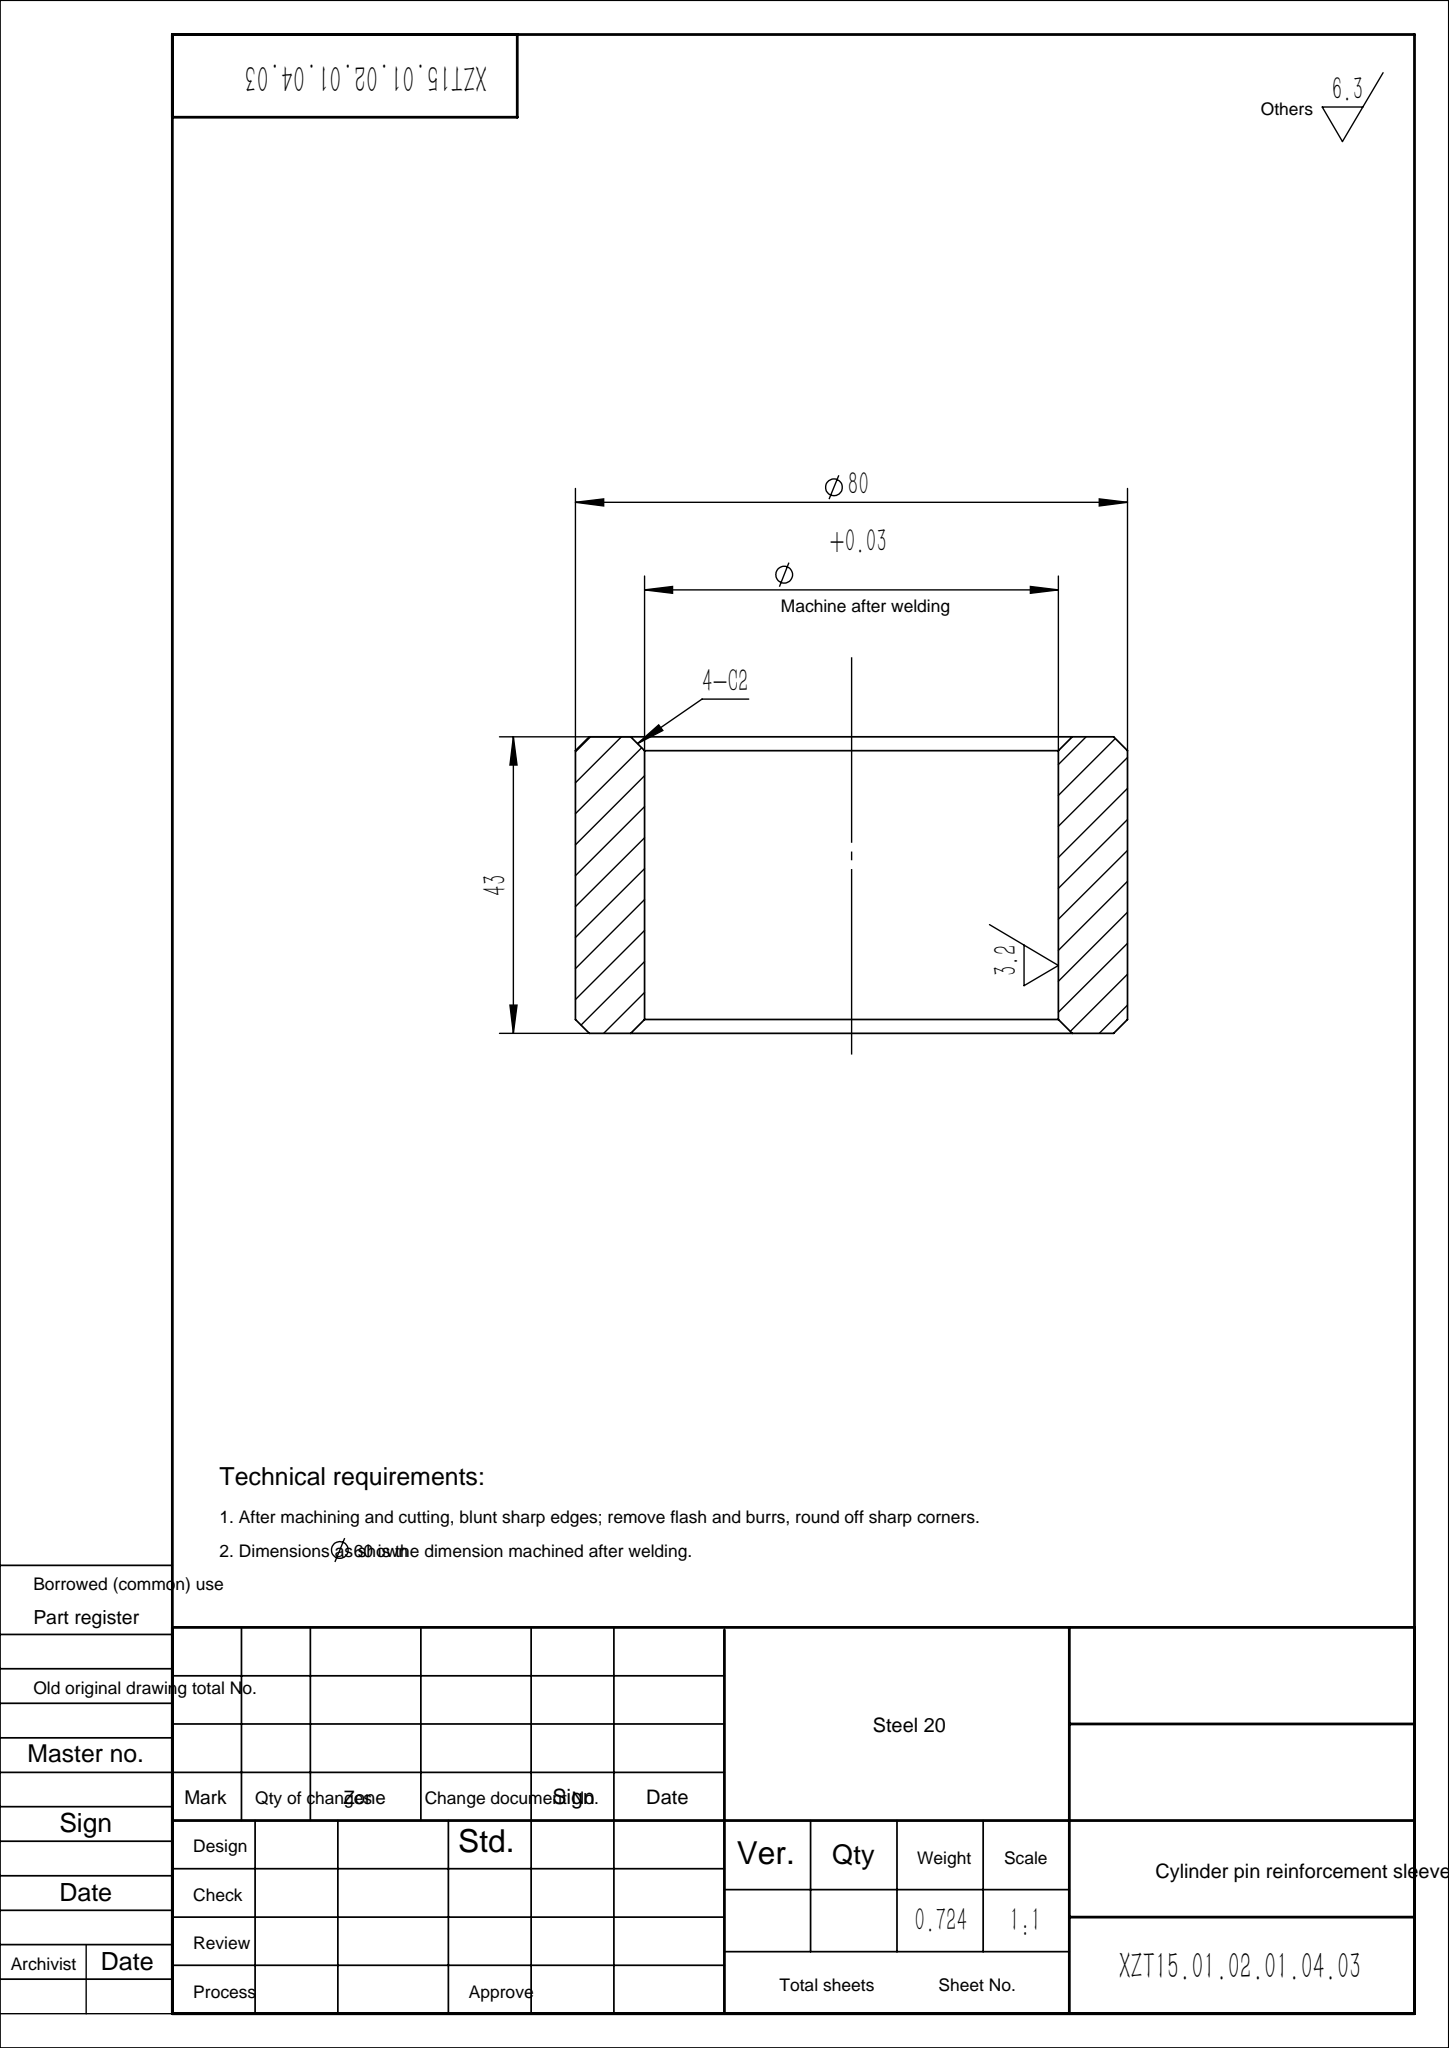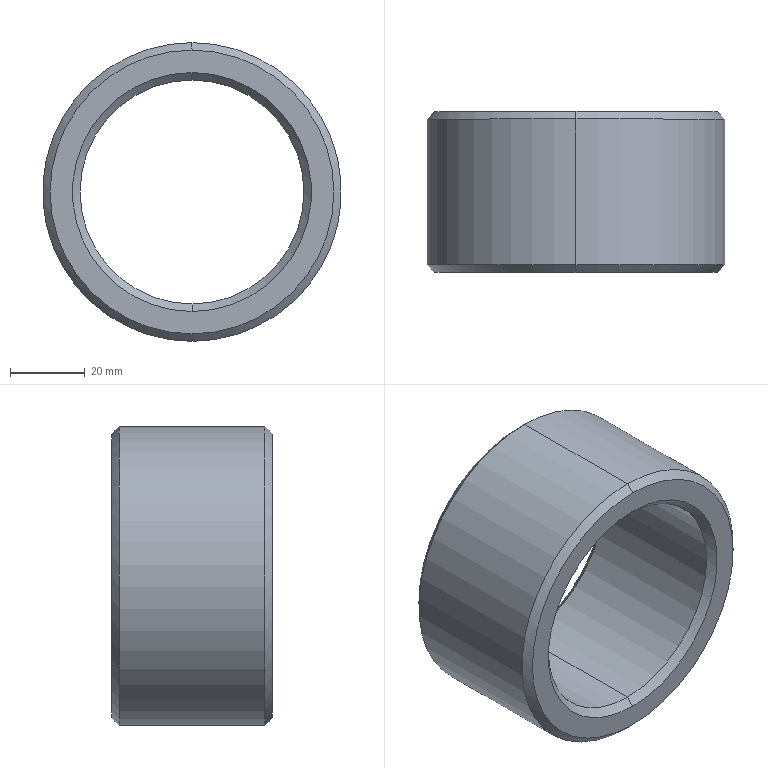Part | SolidWorks | features Chamfer 1, Extrusion 1 | 1 solid | 14 faces | box 80 x 43 x 80 mm | volume 92803 mm3 | cone 8 | cylinder 4 | plane 2 | commonest cylinder face diameters 60 x2 80 x2
STEP:
#1=CARTESIAN_POINT('',(0.,43.,38.));
#2=VERTEX_POINT('',#1);
#3=CARTESIAN_POINT('',(0.,43.,-38.));
#4=VERTEX_POINT('',#3);
#5=CARTESIAN_POINT('',(0.,43.,0.));
#6=DIRECTION('',(0.,1.,0.));
#7=DIRECTION('',(0.,0.,1.));
#8=AXIS2_PLACEMENT_3D('',#5,#6,#7);
#9=CIRCLE('',#8,38.);
#10=EDGE_CURVE('',#2,#4,#9,.T.);
#11=ORIENTED_EDGE('',*,*,#10,.F.);
#12=CARTESIAN_POINT('',(0.,41.,40.));
#13=VERTEX_POINT('',#12);
#14=CARTESIAN_POINT('',(0.,43.,38.));
#15=DIRECTION('',(0.,-0.7071,0.7071));
#16=VECTOR('',#15,1000.);
#17=LINE('',#14,#16);
#18=EDGE_CURVE('',#2,#13,#17,.T.);
#19=ORIENTED_EDGE('',*,*,#18,.T.);
#20=CARTESIAN_POINT('',(0.,41.,-40.));
#21=VERTEX_POINT('',#20);
#22=CARTESIAN_POINT('',(0.,41.,0.));
#23=DIRECTION('',(0.,-1.,0.));
#24=DIRECTION('',(0.,0.,1.));
#25=AXIS2_PLACEMENT_3D('',#22,#23,#24);
#26=CIRCLE('',#25,40.);
#27=EDGE_CURVE('',#21,#13,#26,.T.);
#28=ORIENTED_EDGE('',*,*,#27,.F.);
#29=CARTESIAN_POINT('',(0.,43.,-38.));
#30=DIRECTION('',(0.,-0.7071,-0.7071));
#31=VECTOR('',#30,1000.);
#32=LINE('',#29,#31);
#33=EDGE_CURVE('',#4,#21,#32,.T.);
#34=ORIENTED_EDGE('',*,*,#33,.F.);
#35=EDGE_LOOP('',(#11,#19,#28,#34));
#36=FACE_OUTER_BOUND('',#35,.T.);
#37=CARTESIAN_POINT('',(0.,43.,0.));
#38=DIRECTION('',(0.,-1.,0.));
#39=DIRECTION('',(0.,0.,-1.));
#40=AXIS2_PLACEMENT_3D('',#37,#38,#39);
#41=CONICAL_SURFACE('',#40,38.,0.7854);
#42=ADVANCED_FACE('',(#36),#41,.T.);
#43=CARTESIAN_POINT('',(0.,0.,-38.));
#44=VERTEX_POINT('',#43);
#45=CARTESIAN_POINT('',(0.,0.,38.));
#46=VERTEX_POINT('',#45);
#47=CARTESIAN_POINT('',(0.,0.,0.));
#48=DIRECTION('',(0.,-1.,0.));
#49=DIRECTION('',(0.,0.,1.));
#50=AXIS2_PLACEMENT_3D('',#47,#48,#49);
#51=CIRCLE('',#50,38.);
#52=EDGE_CURVE('',#44,#46,#51,.T.);
#53=ORIENTED_EDGE('',*,*,#52,.F.);
#54=CARTESIAN_POINT('',(0.,2.,-40.));
#55=VERTEX_POINT('',#54);
#56=CARTESIAN_POINT('',(0.,2.,-40.));
#57=DIRECTION('',(0.,0.7071,-0.7071));
#58=VECTOR('',#57,1000.);
#59=LINE('',#56,#58);
#60=EDGE_CURVE('',#44,#55,#59,.T.);
#61=ORIENTED_EDGE('',*,*,#60,.T.);
#62=CARTESIAN_POINT('',(0.,2.,40.));
#63=VERTEX_POINT('',#62);
#64=CARTESIAN_POINT('',(0.,2.,0.));
#65=DIRECTION('',(0.,1.,0.));
#66=DIRECTION('',(0.,0.,1.));
#67=AXIS2_PLACEMENT_3D('',#64,#65,#66);
#68=CIRCLE('',#67,40.);
#69=EDGE_CURVE('',#63,#55,#68,.T.);
#70=ORIENTED_EDGE('',*,*,#69,.F.);
#71=CARTESIAN_POINT('',(0.,2.,40.));
#72=DIRECTION('',(0.,0.7071,0.7071));
#73=VECTOR('',#72,1000.);
#74=LINE('',#71,#73);
#75=EDGE_CURVE('',#46,#63,#74,.T.);
#76=ORIENTED_EDGE('',*,*,#75,.F.);
#77=EDGE_LOOP('',(#53,#61,#70,#76));
#78=FACE_OUTER_BOUND('',#77,.T.);
#79=CARTESIAN_POINT('',(0.,2.,0.));
#80=DIRECTION('',(0.,1.,0.));
#81=DIRECTION('',(0.,0.,1.));
#82=AXIS2_PLACEMENT_3D('',#79,#80,#81);
#83=CONICAL_SURFACE('',#82,40.,0.7854);
#84=ADVANCED_FACE('',(#78),#83,.T.);
#85=CARTESIAN_POINT('',(0.,41.,-30.));
#86=VERTEX_POINT('',#85);
#87=CARTESIAN_POINT('',(0.,41.,30.));
#88=VERTEX_POINT('',#87);
#89=CARTESIAN_POINT('',(0.,41.,0.));
#90=DIRECTION('',(0.,1.,0.));
#91=DIRECTION('',(0.,0.,1.));
#92=AXIS2_PLACEMENT_3D('',#89,#90,#91);
#93=CIRCLE('',#92,30.);
#94=EDGE_CURVE('',#86,#88,#93,.T.);
#95=ORIENTED_EDGE('',*,*,#94,.F.);
#96=CARTESIAN_POINT('',(0.,43.,-32.));
#97=VERTEX_POINT('',#96);
#98=CARTESIAN_POINT('',(0.,41.,-30.));
#99=DIRECTION('',(0.,0.7071,-0.7071));
#100=VECTOR('',#99,1000.);
#101=LINE('',#98,#100);
#102=EDGE_CURVE('',#86,#97,#101,.T.);
#103=ORIENTED_EDGE('',*,*,#102,.T.);
#104=CARTESIAN_POINT('',(0.,43.,32.));
#105=VERTEX_POINT('',#104);
#106=CARTESIAN_POINT('',(0.,43.,0.));
#107=DIRECTION('',(0.,-1.,0.));
#108=DIRECTION('',(0.,0.,1.));
#109=AXIS2_PLACEMENT_3D('',#106,#107,#108);
#110=CIRCLE('',#109,32.);
#111=EDGE_CURVE('',#105,#97,#110,.T.);
#112=ORIENTED_EDGE('',*,*,#111,.F.);
#113=CARTESIAN_POINT('',(0.,41.,30.));
#114=DIRECTION('',(0.,0.7071,0.7071));
#115=VECTOR('',#114,1000.);
#116=LINE('',#113,#115);
#117=EDGE_CURVE('',#88,#105,#116,.T.);
#118=ORIENTED_EDGE('',*,*,#117,.F.);
#119=EDGE_LOOP('',(#95,#103,#112,#118));
#120=FACE_OUTER_BOUND('',#119,.T.);
#121=CARTESIAN_POINT('',(0.,41.,0.));
#122=DIRECTION('',(0.,1.,0.));
#123=DIRECTION('',(0.,0.,1.));
#124=AXIS2_PLACEMENT_3D('',#121,#122,#123);
#125=CONICAL_SURFACE('',#124,30.,0.7854);
#126=ADVANCED_FACE('',(#120),#125,.F.);
#127=CARTESIAN_POINT('',(0.,2.,30.));
#128=VERTEX_POINT('',#127);
#129=CARTESIAN_POINT('',(0.,2.,-30.));
#130=VERTEX_POINT('',#129);
#131=CARTESIAN_POINT('',(0.,2.,0.));
#132=DIRECTION('',(0.,-1.,0.));
#133=DIRECTION('',(0.,0.,1.));
#134=AXIS2_PLACEMENT_3D('',#131,#132,#133);
#135=CIRCLE('',#134,30.);
#136=EDGE_CURVE('',#128,#130,#135,.T.);
#137=ORIENTED_EDGE('',*,*,#136,.F.);
#138=CARTESIAN_POINT('',(0.,0.,32.));
#139=VERTEX_POINT('',#138);
#140=CARTESIAN_POINT('',(0.,0.,32.));
#141=DIRECTION('',(0.,-0.7071,0.7071));
#142=VECTOR('',#141,1000.);
#143=LINE('',#140,#142);
#144=EDGE_CURVE('',#128,#139,#143,.T.);
#145=ORIENTED_EDGE('',*,*,#144,.T.);
#146=CARTESIAN_POINT('',(0.,0.,-32.));
#147=VERTEX_POINT('',#146);
#148=CARTESIAN_POINT('',(0.,0.,0.));
#149=DIRECTION('',(0.,1.,0.));
#150=DIRECTION('',(0.,0.,1.));
#151=AXIS2_PLACEMENT_3D('',#148,#149,#150);
#152=CIRCLE('',#151,32.);
#153=EDGE_CURVE('',#147,#139,#152,.T.);
#154=ORIENTED_EDGE('',*,*,#153,.F.);
#155=CARTESIAN_POINT('',(0.,0.,-32.));
#156=DIRECTION('',(0.,-0.7071,-0.7071));
#157=VECTOR('',#156,1000.);
#158=LINE('',#155,#157);
#159=EDGE_CURVE('',#130,#147,#158,.T.);
#160=ORIENTED_EDGE('',*,*,#159,.F.);
#161=EDGE_LOOP('',(#137,#145,#154,#160));
#162=FACE_OUTER_BOUND('',#161,.T.);
#163=CARTESIAN_POINT('',(0.,0.,0.));
#164=DIRECTION('',(0.,-1.,0.));
#165=DIRECTION('',(0.,0.,-1.));
#166=AXIS2_PLACEMENT_3D('',#163,#164,#165);
#167=CONICAL_SURFACE('',#166,32.,0.7854);
#168=ADVANCED_FACE('',(#162),#167,.F.);
#169=ORIENTED_EDGE('',*,*,#94,.T.);
#170=CARTESIAN_POINT('',(0.,43.,30.));
#171=DIRECTION('',(0.,-1.,0.));
#172=VECTOR('',#171,1000.);
#173=LINE('',#170,#172);
#174=EDGE_CURVE('',#88,#128,#173,.T.);
#175=ORIENTED_EDGE('',*,*,#174,.T.);
#176=ORIENTED_EDGE('',*,*,#136,.T.);
#177=CARTESIAN_POINT('',(0.,43.,-30.));
#178=DIRECTION('',(0.,-1.,0.));
#179=VECTOR('',#178,1000.);
#180=LINE('',#177,#179);
#181=EDGE_CURVE('',#86,#130,#180,.T.);
#182=ORIENTED_EDGE('',*,*,#181,.F.);
#183=EDGE_LOOP('',(#169,#175,#176,#182));
#184=FACE_OUTER_BOUND('',#183,.T.);
#185=CARTESIAN_POINT('',(0.,43.,0.));
#186=DIRECTION('',(0.,-1.,0.));
#187=DIRECTION('',(0.,0.,-1.));
#188=AXIS2_PLACEMENT_3D('',#185,#186,#187);
#189=CYLINDRICAL_SURFACE('',#188,30.);
#190=ADVANCED_FACE('',(#184),#189,.F.);
#191=ORIENTED_EDGE('',*,*,#27,.T.);
#192=CARTESIAN_POINT('',(0.,43.,40.));
#193=DIRECTION('',(0.,-1.,0.));
#194=VECTOR('',#193,1000.);
#195=LINE('',#192,#194);
#196=EDGE_CURVE('',#13,#63,#195,.T.);
#197=ORIENTED_EDGE('',*,*,#196,.T.);
#198=ORIENTED_EDGE('',*,*,#69,.T.);
#199=CARTESIAN_POINT('',(0.,43.,-40.));
#200=DIRECTION('',(0.,-1.,0.));
#201=VECTOR('',#200,1000.);
#202=LINE('',#199,#201);
#203=EDGE_CURVE('',#21,#55,#202,.T.);
#204=ORIENTED_EDGE('',*,*,#203,.F.);
#205=EDGE_LOOP('',(#191,#197,#198,#204));
#206=FACE_OUTER_BOUND('',#205,.T.);
#207=CARTESIAN_POINT('',(0.,43.,0.));
#208=DIRECTION('',(0.,-1.,0.));
#209=DIRECTION('',(0.,0.,-1.));
#210=AXIS2_PLACEMENT_3D('',#207,#208,#209);
#211=CYLINDRICAL_SURFACE('',#210,40.);
#212=ADVANCED_FACE('',(#206),#211,.T.);
#213=ORIENTED_EDGE('',*,*,#111,.T.);
#214=CARTESIAN_POINT('',(0.,43.,0.));
#215=DIRECTION('',(0.,-1.,0.));
#216=DIRECTION('',(0.,0.,1.));
#217=AXIS2_PLACEMENT_3D('',#214,#215,#216);
#218=CIRCLE('',#217,32.);
#219=EDGE_CURVE('',#97,#105,#218,.T.);
#220=ORIENTED_EDGE('',*,*,#219,.T.);
#221=EDGE_LOOP('',(#213,#220));
#222=FACE_BOUND('',#221,.T.);
#223=CARTESIAN_POINT('',(0.,43.,0.));
#224=DIRECTION('',(0.,1.,0.));
#225=DIRECTION('',(0.,0.,1.));
#226=AXIS2_PLACEMENT_3D('',#223,#224,#225);
#227=CIRCLE('',#226,38.);
#228=EDGE_CURVE('',#4,#2,#227,.T.);
#229=ORIENTED_EDGE('',*,*,#228,.T.);
#230=ORIENTED_EDGE('',*,*,#10,.T.);
#231=EDGE_LOOP('',(#229,#230));
#232=FACE_OUTER_BOUND('',#231,.T.);
#233=CARTESIAN_POINT('',(0.,43.,0.));
#234=DIRECTION('',(0.,1.,0.));
#235=DIRECTION('',(0.,0.,1.));
#236=AXIS2_PLACEMENT_3D('',#233,#234,#235);
#237=PLANE('',#236);
#238=ADVANCED_FACE('',(#222,#232),#237,.T.);
#239=ORIENTED_EDGE('',*,*,#153,.T.);
#240=CARTESIAN_POINT('',(0.,0.,0.));
#241=DIRECTION('',(0.,1.,0.));
#242=DIRECTION('',(0.,0.,1.));
#243=AXIS2_PLACEMENT_3D('',#240,#241,#242);
#244=CIRCLE('',#243,32.);
#245=EDGE_CURVE('',#139,#147,#244,.T.);
#246=ORIENTED_EDGE('',*,*,#245,.T.);
#247=EDGE_LOOP('',(#239,#246));
#248=FACE_BOUND('',#247,.T.);
#249=CARTESIAN_POINT('',(0.,0.,0.));
#250=DIRECTION('',(0.,-1.,0.));
#251=DIRECTION('',(0.,0.,1.));
#252=AXIS2_PLACEMENT_3D('',#249,#250,#251);
#253=CIRCLE('',#252,38.);
#254=EDGE_CURVE('',#46,#44,#253,.T.);
#255=ORIENTED_EDGE('',*,*,#254,.T.);
#256=ORIENTED_EDGE('',*,*,#52,.T.);
#257=EDGE_LOOP('',(#255,#256));
#258=FACE_OUTER_BOUND('',#257,.T.);
#259=CARTESIAN_POINT('',(0.,0.,0.));
#260=DIRECTION('',(0.,1.,0.));
#261=DIRECTION('',(0.,0.,1.));
#262=AXIS2_PLACEMENT_3D('',#259,#260,#261);
#263=PLANE('',#262);
#264=ADVANCED_FACE('',(#248,#258),#263,.F.);
#265=ORIENTED_EDGE('',*,*,#196,.F.);
#266=CARTESIAN_POINT('',(0.,41.,0.));
#267=DIRECTION('',(0.,-1.,0.));
#268=DIRECTION('',(0.,0.,1.));
#269=AXIS2_PLACEMENT_3D('',#266,#267,#268);
#270=CIRCLE('',#269,40.);
#271=EDGE_CURVE('',#13,#21,#270,.T.);
#272=ORIENTED_EDGE('',*,*,#271,.T.);
#273=ORIENTED_EDGE('',*,*,#203,.T.);
#274=CARTESIAN_POINT('',(0.,2.,0.));
#275=DIRECTION('',(0.,1.,0.));
#276=DIRECTION('',(0.,0.,1.));
#277=AXIS2_PLACEMENT_3D('',#274,#275,#276);
#278=CIRCLE('',#277,40.);
#279=EDGE_CURVE('',#55,#63,#278,.T.);
#280=ORIENTED_EDGE('',*,*,#279,.T.);
#281=EDGE_LOOP('',(#265,#272,#273,#280));
#282=FACE_OUTER_BOUND('',#281,.T.);
#283=CARTESIAN_POINT('',(0.,43.,0.));
#284=DIRECTION('',(0.,-1.,0.));
#285=DIRECTION('',(0.,0.,-1.));
#286=AXIS2_PLACEMENT_3D('',#283,#284,#285);
#287=CYLINDRICAL_SURFACE('',#286,40.);
#288=ADVANCED_FACE('',(#282),#287,.T.);
#289=ORIENTED_EDGE('',*,*,#174,.F.);
#290=CARTESIAN_POINT('',(0.,41.,0.));
#291=DIRECTION('',(0.,1.,0.));
#292=DIRECTION('',(0.,0.,1.));
#293=AXIS2_PLACEMENT_3D('',#290,#291,#292);
#294=CIRCLE('',#293,30.);
#295=EDGE_CURVE('',#88,#86,#294,.T.);
#296=ORIENTED_EDGE('',*,*,#295,.T.);
#297=ORIENTED_EDGE('',*,*,#181,.T.);
#298=CARTESIAN_POINT('',(0.,2.,0.));
#299=DIRECTION('',(0.,-1.,0.));
#300=DIRECTION('',(0.,0.,1.));
#301=AXIS2_PLACEMENT_3D('',#298,#299,#300);
#302=CIRCLE('',#301,30.);
#303=EDGE_CURVE('',#130,#128,#302,.T.);
#304=ORIENTED_EDGE('',*,*,#303,.T.);
#305=EDGE_LOOP('',(#289,#296,#297,#304));
#306=FACE_OUTER_BOUND('',#305,.T.);
#307=CARTESIAN_POINT('',(0.,43.,0.));
#308=DIRECTION('',(0.,-1.,0.));
#309=DIRECTION('',(0.,0.,-1.));
#310=AXIS2_PLACEMENT_3D('',#307,#308,#309);
#311=CYLINDRICAL_SURFACE('',#310,30.);
#312=ADVANCED_FACE('',(#306),#311,.F.);
#313=ORIENTED_EDGE('',*,*,#144,.F.);
#314=ORIENTED_EDGE('',*,*,#303,.F.);
#315=ORIENTED_EDGE('',*,*,#159,.T.);
#316=ORIENTED_EDGE('',*,*,#245,.F.);
#317=EDGE_LOOP('',(#313,#314,#315,#316));
#318=FACE_OUTER_BOUND('',#317,.T.);
#319=CARTESIAN_POINT('',(0.,0.,0.));
#320=DIRECTION('',(0.,-1.,0.));
#321=DIRECTION('',(0.,0.,-1.));
#322=AXIS2_PLACEMENT_3D('',#319,#320,#321);
#323=CONICAL_SURFACE('',#322,32.,0.7854);
#324=ADVANCED_FACE('',(#318),#323,.F.);
#325=ORIENTED_EDGE('',*,*,#102,.F.);
#326=ORIENTED_EDGE('',*,*,#295,.F.);
#327=ORIENTED_EDGE('',*,*,#117,.T.);
#328=ORIENTED_EDGE('',*,*,#219,.F.);
#329=EDGE_LOOP('',(#325,#326,#327,#328));
#330=FACE_OUTER_BOUND('',#329,.T.);
#331=CARTESIAN_POINT('',(0.,41.,0.));
#332=DIRECTION('',(0.,1.,0.));
#333=DIRECTION('',(0.,0.,1.));
#334=AXIS2_PLACEMENT_3D('',#331,#332,#333);
#335=CONICAL_SURFACE('',#334,30.,0.7854);
#336=ADVANCED_FACE('',(#330),#335,.F.);
#337=ORIENTED_EDGE('',*,*,#60,.F.);
#338=ORIENTED_EDGE('',*,*,#254,.F.);
#339=ORIENTED_EDGE('',*,*,#75,.T.);
#340=ORIENTED_EDGE('',*,*,#279,.F.);
#341=EDGE_LOOP('',(#337,#338,#339,#340));
#342=FACE_OUTER_BOUND('',#341,.T.);
#343=CARTESIAN_POINT('',(0.,2.,0.));
#344=DIRECTION('',(0.,1.,0.));
#345=DIRECTION('',(0.,0.,1.));
#346=AXIS2_PLACEMENT_3D('',#343,#344,#345);
#347=CONICAL_SURFACE('',#346,40.,0.7854);
#348=ADVANCED_FACE('',(#342),#347,.T.);
#349=ORIENTED_EDGE('',*,*,#18,.F.);
#350=ORIENTED_EDGE('',*,*,#228,.F.);
#351=ORIENTED_EDGE('',*,*,#33,.T.);
#352=ORIENTED_EDGE('',*,*,#271,.F.);
#353=EDGE_LOOP('',(#349,#350,#351,#352));
#354=FACE_OUTER_BOUND('',#353,.T.);
#355=CARTESIAN_POINT('',(0.,43.,0.));
#356=DIRECTION('',(0.,-1.,0.));
#357=DIRECTION('',(0.,0.,-1.));
#358=AXIS2_PLACEMENT_3D('',#355,#356,#357);
#359=CONICAL_SURFACE('',#358,38.,0.7854);
#360=ADVANCED_FACE('',(#354),#359,.T.);
#361=CLOSED_SHELL('',(#42,#84,#126,#168,#190,#212,#238,#264,#288,#312,#324,#336,#348,#360));
#362=MANIFOLD_SOLID_BREP('',#361);
#363=CARTESIAN_POINT('',(0.,0.,0.));
#364=DIRECTION('',(0.,0.,1.));
#365=DIRECTION('',(1.,0.,0.));
#366=AXIS2_PLACEMENT_3D('',#363,#364,#365);
#367=(LENGTH_UNIT()NAMED_UNIT(*)SI_UNIT(.MILLI.,.METRE.));
#368=UNCERTAINTY_MEASURE_WITH_UNIT(LENGTH_MEASURE(0.00001),#367,'','');
#369=(NAMED_UNIT(*)PLANE_ANGLE_UNIT()SI_UNIT($,.RADIAN.));
#370=(NAMED_UNIT(*)SI_UNIT($,.STERADIAN.)SOLID_ANGLE_UNIT());
#371=(GEOMETRIC_REPRESENTATION_CONTEXT(3)GLOBAL_UNCERTAINTY_ASSIGNED_CONTEXT((#368))GLOBAL_UNIT_ASSIGNED_CONTEXT((#367,#369,#370))REPRESENTATION_CONTEXT('',''));
#372=ADVANCED_BREP_SHAPE_REPRESENTATION('',(#362,#366),#371);